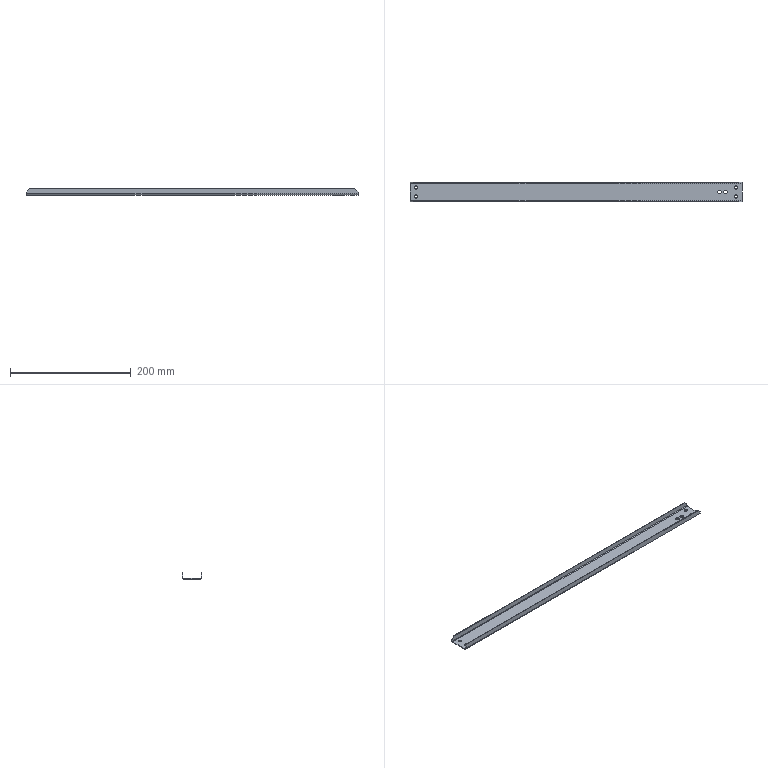Part | STEP file | ASND-0110-Body 1-6 | 1 solid | 38 faces | box 550 x 32 x 10 mm | volume 26590 mm3 | plane 22 | cylinder 16 | commonest cylinder face diameters 5.5 x8 6 x4 2 x2 4 x2